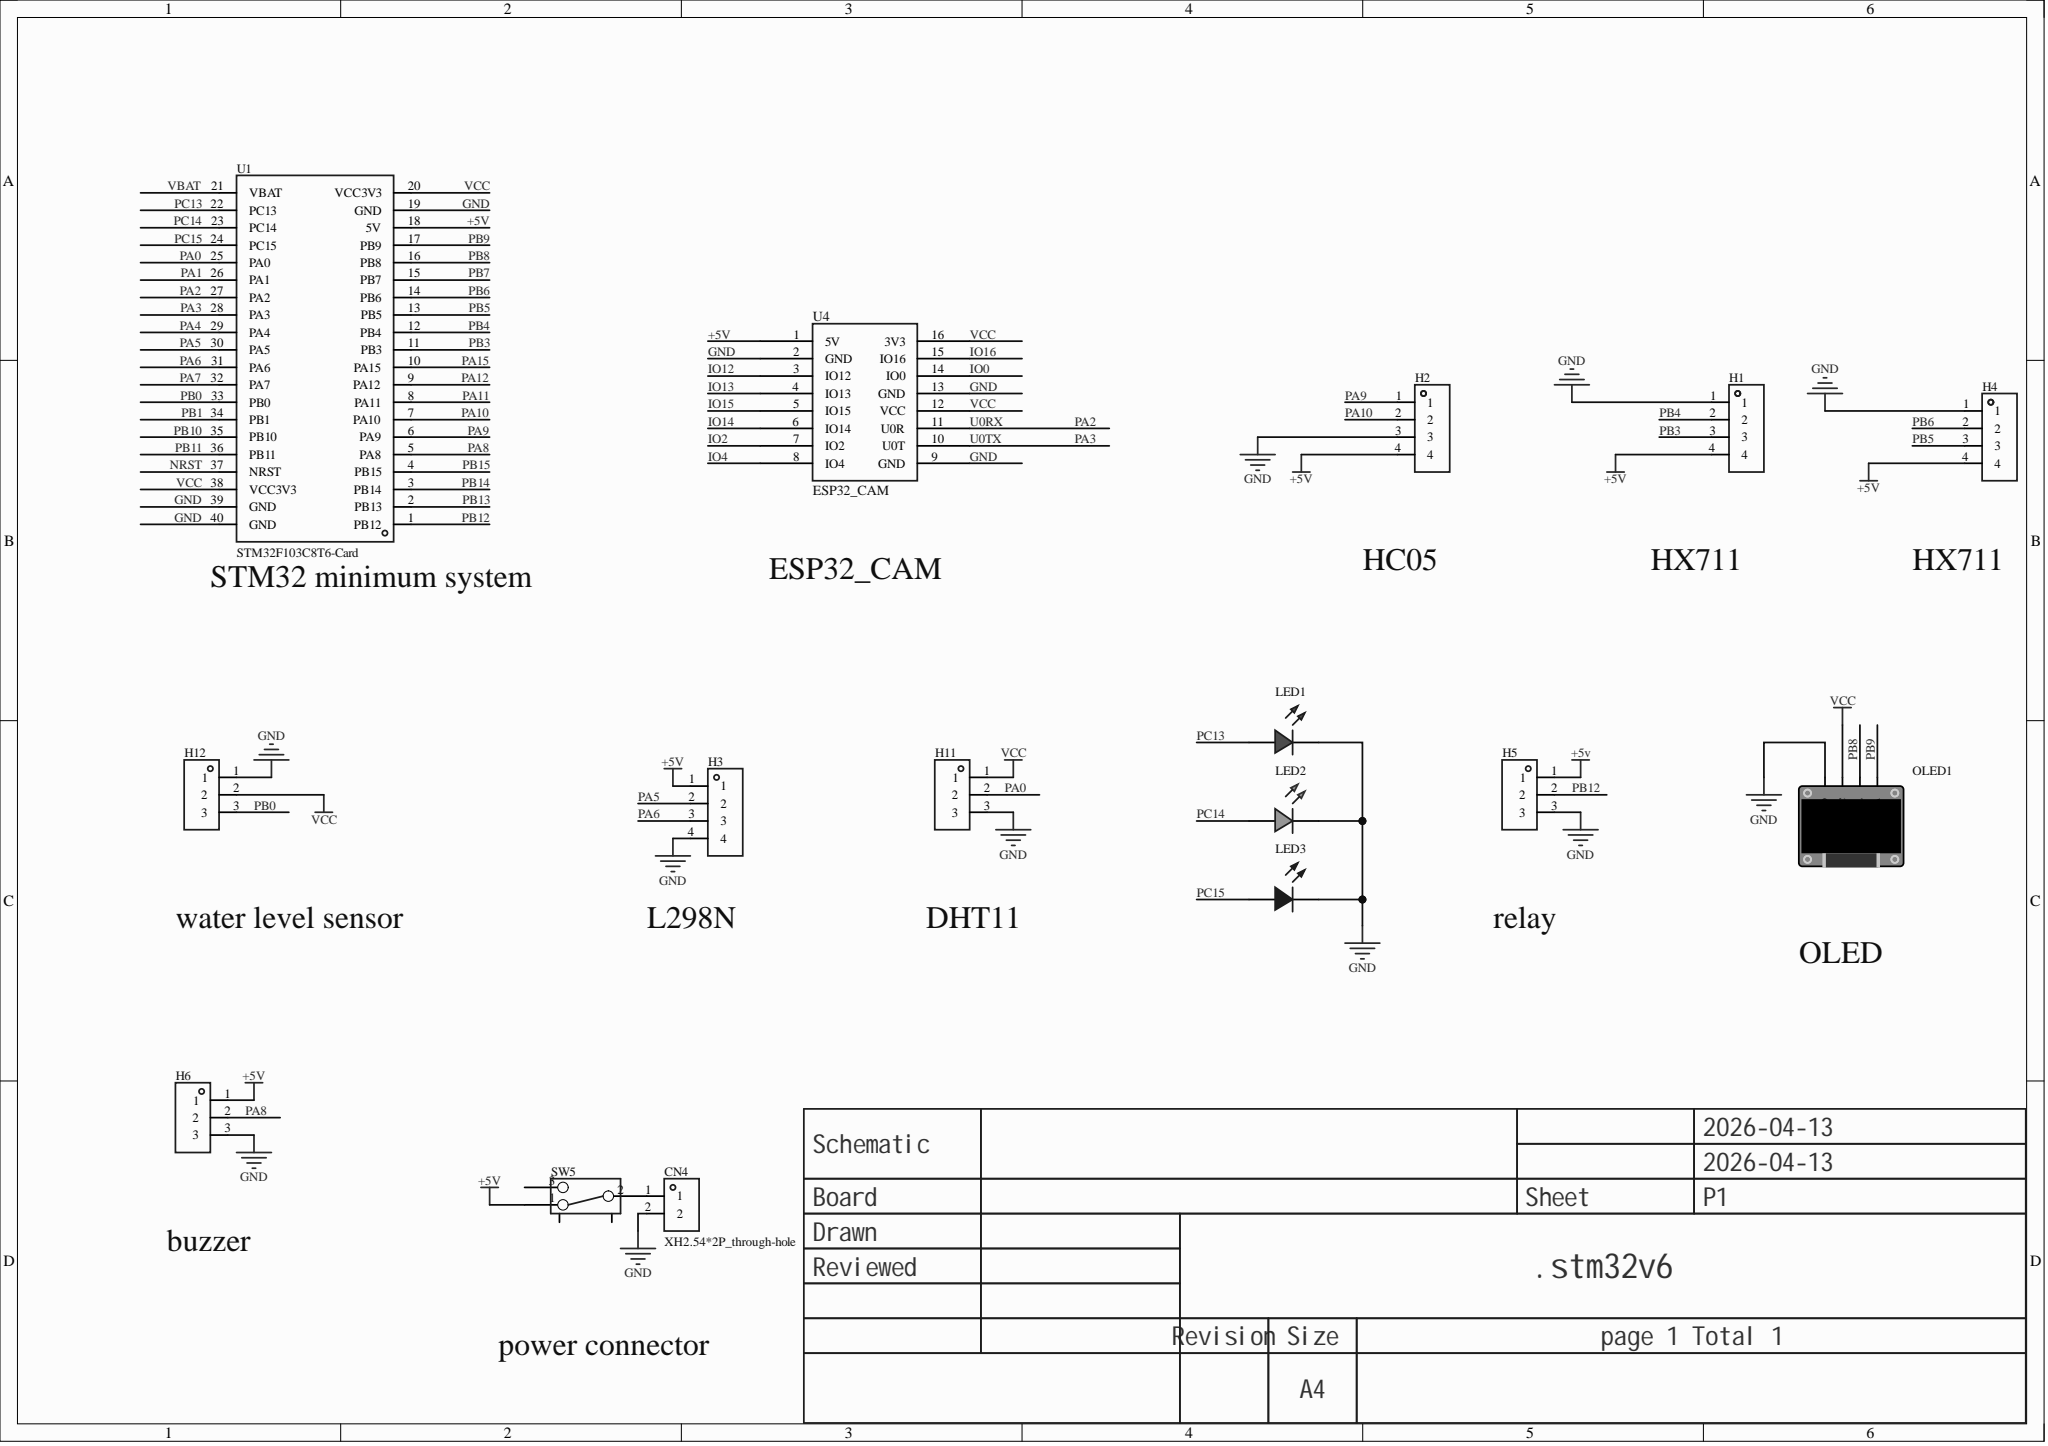Circuit board | Altium Designer | 16 parts | 23 nets
Bill of materials:
Comment,Description,Designator,Footprint,LibRef,Quantity
"XH2.54*2P_through-hole","","CN4","CONN-TH_2P-P2.50-XH2.54-2P","XH2.54*2P_直插","1"
"","","H1, H2, H4","HDR-TH_4P-P2.54-V-F","HDR-F_2.54_1x4P","3"
"","","H3","HDR-TH_4P-P2.54-V-M","HDR-M_2.54_1x4P","1"
"","","H5, H6, H11, H12","HDR-TH_3P-P2.54-V-F","HDR-F_2.54_1x3P","4"
"","","LED1, LED2, LED3","LED_TH-3mm","LED_TH-R_3mm, LED_TH-G_3mm, LED_TH-B_3mm","3"
"","","OLED1","0.96OLED_4P","0.96OLED模块_4P","1"
"","","SW5","拨动开关","拨动开关_正","1"
"STM32F103C8T6-Card","","U1","CONN-TH_L53.3-W22.9_STM32F103C8T6-CARD","STM32F103C8T6-Card","1"
"ESP32_CAM","ESP32-CAM module","U4","ESP32-CAM","ESP32_CAM","1"
Netlist (Protel format):
[
CN4
CONN-TH_2P-P2.50-XH2.54-2P
XH2.54*2P_through-hole



]
[
H1
HDR-TH_4P-P2.54-V-F




]
[
H2
HDR-TH_4P-P2.54-V-F




]
[
H3
HDR-TH_4P-P2.54-V-M




]
[
H4
HDR-TH_4P-P2.54-V-F




]
[
H5
HDR-TH_3P-P2.54-V-F




]
[
H6
HDR-TH_3P-P2.54-V-F




]
[
H11
HDR-TH_3P-P2.54-V-F




]
[
H12
HDR-TH_3P-P2.54-V-F




]
[
LED1
LED_TH-3mm




]
[
LED2
LED_TH-3mm




]
[
LED3
LED_TH-3mm




]
[
OLED1
0.96OLED_4P




]
[
SW5
拨动开关




]
[
U1
CONN-TH_L53.3-W22.9_STM32F103C8T6-CARD
STM32F103C8T6-Card



]
[
U4
ESP32-CAM
ESP32_CAM



]
(
VCC
H11-1
H12-2
OLED1-2
U1-20
U1-38
U4-12
U4-16
)
(
PC15
LED3-1
U1-24
)
(
PC14
LED2-1
U1-23
)
(
PC13
LED1-1
U1-22
)
(
PB12
H5-2
U1-1
)
(
PB9
OLED1-4
U1-17
)
(
PB8
OLED1-3
U1-16
)
(
PB6
H4-2
U1-14
)
(
PB5
H4-3
U1-13
)
(
PB4
H1-2
U1-12
)
(
PB3
H1-3
U1-11
)
(
PB0
H12-3
U1-33
)
(
PA10
H2-2
U1-7
)
(
PA9
H2-1
U1-6
)
(
PA8
H6-2
U1-5
)
(
PA6
H3-3
U1-31
)
(
PA5
H3-2
U1-30
)
(
PA3
U1-28
U4-10
)
(
PA2
U1-27
U4-11
)
(
PA0
H11-2
U1-25
)
(
NetCN4_1
CN4-1
SW5-2
)
(
GND
CN4-2
H1-1
H2-3
H3-4
H4-1
H5-3
H6-3
H11-3
H12-1
LED1-2
LED2-2
LED3-2
OLED1-1
U1-19
U1-39
U1-40
U4-2
U4-9
U4-13
)
(
+5V
H1-4
H2-4
H3-1
H4-4
H5-1
H6-1
SW5-1
U1-18
U4-1
)